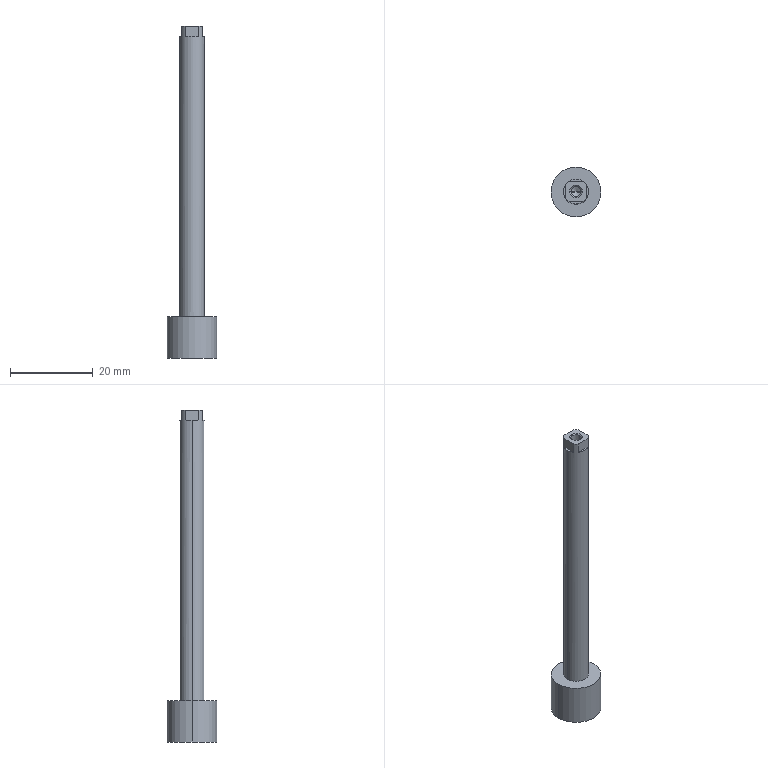Part | SolidWorks | features BaseBody 1 | 1 solid | 21 faces | box 12 x 12 x 80 mm | volume 3071 mm3 | plane 11 | cylinder 6 | cone 4 | commonest cylinder face diameters 2.459 x2 6 x2 12 x2
STEP:
#1=CARTESIAN_POINT('',(3.,0.,-37.5));
#2=VERTEX_POINT('',#1);
#3=CARTESIAN_POINT('',(-3.,0.,-37.5));
#4=VERTEX_POINT('',#3);
#5=CARTESIAN_POINT('',(0.,0.,-37.5));
#6=DIRECTION('',(0.,0.,1.));
#7=DIRECTION('',(1.,0.,0.));
#8=AXIS2_PLACEMENT_3D('',#5,#6,#7);
#9=CIRCLE('',#8,3.);
#10=EDGE_CURVE('',#2,#4,#9,.T.);
#11=ORIENTED_EDGE('',*,*,#10,.T.);
#12=CARTESIAN_POINT('',(-3.,0.,30.));
#13=VERTEX_POINT('',#12);
#14=CARTESIAN_POINT('',(-3.,0.,-2.5));
#15=DIRECTION('',(0.,0.,1.));
#16=VECTOR('',#15,1000.);
#17=LINE('',#14,#16);
#18=EDGE_CURVE('',#4,#13,#17,.T.);
#19=ORIENTED_EDGE('',*,*,#18,.T.);
#20=CARTESIAN_POINT('',(-2.5,1.658,30.));
#21=VERTEX_POINT('',#20);
#22=CARTESIAN_POINT('',(0.,0.,30.));
#23=DIRECTION('',(0.,0.,-1.));
#24=DIRECTION('',(1.,0.,0.));
#25=AXIS2_PLACEMENT_3D('',#22,#23,#24);
#26=CIRCLE('',#25,3.);
#27=EDGE_CURVE('',#13,#21,#26,.T.);
#28=ORIENTED_EDGE('',*,*,#27,.T.);
#29=CARTESIAN_POINT('',(-2.5,1.658,32.5));
#30=VERTEX_POINT('',#29);
#31=CARTESIAN_POINT('',(-2.5,1.658,-2.5));
#32=DIRECTION('',(0.,0.,1.));
#33=VECTOR('',#32,1000.);
#34=LINE('',#31,#33);
#35=EDGE_CURVE('',#21,#30,#34,.T.);
#36=ORIENTED_EDGE('',*,*,#35,.T.);
#37=CARTESIAN_POINT('',(-1.658,2.5,32.5));
#38=VERTEX_POINT('',#37);
#39=CARTESIAN_POINT('',(0.,0.,32.5));
#40=DIRECTION('',(0.,0.,1.));
#41=DIRECTION('',(1.,0.,0.));
#42=AXIS2_PLACEMENT_3D('',#39,#40,#41);
#43=CIRCLE('',#42,3.);
#44=EDGE_CURVE('',#38,#30,#43,.T.);
#45=ORIENTED_EDGE('',*,*,#44,.F.);
#46=CARTESIAN_POINT('',(-1.658,2.5,30.));
#47=VERTEX_POINT('',#46);
#48=CARTESIAN_POINT('',(-1.658,2.5,-2.5));
#49=DIRECTION('',(0.,0.,-1.));
#50=VECTOR('',#49,1000.);
#51=LINE('',#48,#50);
#52=EDGE_CURVE('',#38,#47,#51,.T.);
#53=ORIENTED_EDGE('',*,*,#52,.T.);
#54=CARTESIAN_POINT('',(1.658,2.5,30.));
#55=VERTEX_POINT('',#54);
#56=CARTESIAN_POINT('',(0.,0.,30.));
#57=DIRECTION('',(0.,0.,-1.));
#58=DIRECTION('',(1.,0.,0.));
#59=AXIS2_PLACEMENT_3D('',#56,#57,#58);
#60=CIRCLE('',#59,3.);
#61=EDGE_CURVE('',#47,#55,#60,.T.);
#62=ORIENTED_EDGE('',*,*,#61,.T.);
#63=CARTESIAN_POINT('',(1.658,2.5,32.5));
#64=VERTEX_POINT('',#63);
#65=CARTESIAN_POINT('',(1.658,2.5,-2.5));
#66=DIRECTION('',(0.,0.,1.));
#67=VECTOR('',#66,1000.);
#68=LINE('',#65,#67);
#69=EDGE_CURVE('',#55,#64,#68,.T.);
#70=ORIENTED_EDGE('',*,*,#69,.T.);
#71=CARTESIAN_POINT('',(2.5,1.658,32.5));
#72=VERTEX_POINT('',#71);
#73=CARTESIAN_POINT('',(0.,0.,32.5));
#74=DIRECTION('',(0.,0.,1.));
#75=DIRECTION('',(1.,0.,0.));
#76=AXIS2_PLACEMENT_3D('',#73,#74,#75);
#77=CIRCLE('',#76,3.);
#78=EDGE_CURVE('',#72,#64,#77,.T.);
#79=ORIENTED_EDGE('',*,*,#78,.F.);
#80=CARTESIAN_POINT('',(2.5,1.658,30.));
#81=VERTEX_POINT('',#80);
#82=CARTESIAN_POINT('',(2.5,1.658,-2.5));
#83=DIRECTION('',(0.,0.,-1.));
#84=VECTOR('',#83,1000.);
#85=LINE('',#82,#84);
#86=EDGE_CURVE('',#72,#81,#85,.T.);
#87=ORIENTED_EDGE('',*,*,#86,.T.);
#88=CARTESIAN_POINT('',(3.,0.,30.));
#89=VERTEX_POINT('',#88);
#90=CARTESIAN_POINT('',(0.,0.,30.));
#91=DIRECTION('',(0.,0.,-1.));
#92=DIRECTION('',(1.,0.,0.));
#93=AXIS2_PLACEMENT_3D('',#90,#91,#92);
#94=CIRCLE('',#93,3.);
#95=EDGE_CURVE('',#81,#89,#94,.T.);
#96=ORIENTED_EDGE('',*,*,#95,.T.);
#97=CARTESIAN_POINT('',(3.,0.,-2.5));
#98=DIRECTION('',(0.,0.,1.));
#99=VECTOR('',#98,1000.);
#100=LINE('',#97,#99);
#101=EDGE_CURVE('',#2,#89,#100,.T.);
#102=ORIENTED_EDGE('',*,*,#101,.F.);
#103=EDGE_LOOP('',(#11,#19,#28,#36,#45,#53,#62,#70,#79,#87,#96,#102));
#104=FACE_OUTER_BOUND('',#103,.T.);
#105=CARTESIAN_POINT('',(0.,0.,-2.5));
#106=DIRECTION('',(0.,0.,1.));
#107=DIRECTION('',(1.,0.,0.));
#108=AXIS2_PLACEMENT_3D('',#105,#106,#107);
#109=CYLINDRICAL_SURFACE('',#108,3.);
#110=ADVANCED_FACE('',(#104),#109,.T.);
#111=CARTESIAN_POINT('',(6.,0.,-47.5));
#112=VERTEX_POINT('',#111);
#113=CARTESIAN_POINT('',(-6.,0.,-47.5));
#114=VERTEX_POINT('',#113);
#115=CARTESIAN_POINT('',(0.,0.,-47.5));
#116=DIRECTION('',(0.,0.,1.));
#117=DIRECTION('',(1.,0.,0.));
#118=AXIS2_PLACEMENT_3D('',#115,#116,#117);
#119=CIRCLE('',#118,6.);
#120=EDGE_CURVE('',#112,#114,#119,.T.);
#121=ORIENTED_EDGE('',*,*,#120,.T.);
#122=CARTESIAN_POINT('',(-6.,0.,-37.5));
#123=VERTEX_POINT('',#122);
#124=CARTESIAN_POINT('',(-6.,0.,-42.5));
#125=DIRECTION('',(0.,0.,1.));
#126=VECTOR('',#125,1000.);
#127=LINE('',#124,#126);
#128=EDGE_CURVE('',#114,#123,#127,.T.);
#129=ORIENTED_EDGE('',*,*,#128,.T.);
#130=CARTESIAN_POINT('',(6.,0.,-37.5));
#131=VERTEX_POINT('',#130);
#132=CARTESIAN_POINT('',(0.,0.,-37.5));
#133=DIRECTION('',(0.,0.,1.));
#134=DIRECTION('',(1.,0.,0.));
#135=AXIS2_PLACEMENT_3D('',#132,#133,#134);
#136=CIRCLE('',#135,6.);
#137=EDGE_CURVE('',#131,#123,#136,.T.);
#138=ORIENTED_EDGE('',*,*,#137,.F.);
#139=CARTESIAN_POINT('',(6.,0.,-42.5));
#140=DIRECTION('',(0.,0.,1.));
#141=VECTOR('',#140,1000.);
#142=LINE('',#139,#141);
#143=EDGE_CURVE('',#112,#131,#142,.T.);
#144=ORIENTED_EDGE('',*,*,#143,.F.);
#145=EDGE_LOOP('',(#121,#129,#138,#144));
#146=FACE_OUTER_BOUND('',#145,.T.);
#147=CARTESIAN_POINT('',(0.,0.,-42.5));
#148=DIRECTION('',(0.,0.,1.));
#149=DIRECTION('',(1.,0.,0.));
#150=AXIS2_PLACEMENT_3D('',#147,#148,#149);
#151=CYLINDRICAL_SURFACE('',#150,6.);
#152=ADVANCED_FACE('',(#146),#151,.T.);
#153=CARTESIAN_POINT('',(-1.23,0.,32.23));
#154=VERTEX_POINT('',#153);
#155=CARTESIAN_POINT('',(1.23,0.,32.23));
#156=VERTEX_POINT('',#155);
#157=CARTESIAN_POINT('',(0.,0.,32.23));
#158=DIRECTION('',(0.,0.,1.));
#159=DIRECTION('',(1.,0.,0.));
#160=AXIS2_PLACEMENT_3D('',#157,#158,#159);
#161=CIRCLE('',#160,1.23);
#162=EDGE_CURVE('',#154,#156,#161,.T.);
#163=ORIENTED_EDGE('',*,*,#162,.F.);
#164=CARTESIAN_POINT('',(-1.5,0.,32.5));
#165=VERTEX_POINT('',#164);
#166=CARTESIAN_POINT('',(-1.5,0.,32.5));
#167=DIRECTION('',(-0.7071,0.,0.7071));
#168=VECTOR('',#167,1000.);
#169=LINE('',#166,#168);
#170=EDGE_CURVE('',#154,#165,#169,.T.);
#171=ORIENTED_EDGE('',*,*,#170,.T.);
#172=CARTESIAN_POINT('',(1.5,0.,32.5));
#173=VERTEX_POINT('',#172);
#174=CARTESIAN_POINT('',(0.,0.,32.5));
#175=DIRECTION('',(0.,0.,-1.));
#176=DIRECTION('',(1.,0.,0.));
#177=AXIS2_PLACEMENT_3D('',#174,#175,#176);
#178=CIRCLE('',#177,1.5);
#179=EDGE_CURVE('',#173,#165,#178,.T.);
#180=ORIENTED_EDGE('',*,*,#179,.F.);
#181=CARTESIAN_POINT('',(1.5,0.,32.5));
#182=DIRECTION('',(0.7071,0.,0.7071));
#183=VECTOR('',#182,1000.);
#184=LINE('',#181,#183);
#185=EDGE_CURVE('',#156,#173,#184,.T.);
#186=ORIENTED_EDGE('',*,*,#185,.F.);
#187=EDGE_LOOP('',(#163,#171,#180,#186));
#188=FACE_OUTER_BOUND('',#187,.T.);
#189=CARTESIAN_POINT('',(0.,0.,32.5));
#190=DIRECTION('',(0.,0.,1.));
#191=DIRECTION('',(1.,0.,0.));
#192=AXIS2_PLACEMENT_3D('',#189,#190,#191);
#193=CONICAL_SURFACE('',#192,1.5,0.7854);
#194=ADVANCED_FACE('',(#188),#193,.F.);
#195=CARTESIAN_POINT('',(-1.23,0.,27.));
#196=VERTEX_POINT('',#195);
#197=CARTESIAN_POINT('',(1.23,0.,27.));
#198=VERTEX_POINT('',#197);
#199=CARTESIAN_POINT('',(0.,0.,27.));
#200=DIRECTION('',(0.,0.,1.));
#201=DIRECTION('',(1.,0.,0.));
#202=AXIS2_PLACEMENT_3D('',#199,#200,#201);
#203=CIRCLE('',#202,1.23);
#204=EDGE_CURVE('',#196,#198,#203,.T.);
#205=ORIENTED_EDGE('',*,*,#204,.F.);
#206=CARTESIAN_POINT('',(-1.23,0.,29.615));
#207=DIRECTION('',(0.,0.,1.));
#208=VECTOR('',#207,1000.);
#209=LINE('',#206,#208);
#210=EDGE_CURVE('',#196,#154,#209,.T.);
#211=ORIENTED_EDGE('',*,*,#210,.T.);
#212=ORIENTED_EDGE('',*,*,#162,.T.);
#213=CARTESIAN_POINT('',(1.23,0.,29.615));
#214=DIRECTION('',(0.,0.,1.));
#215=VECTOR('',#214,1000.);
#216=LINE('',#213,#215);
#217=EDGE_CURVE('',#198,#156,#216,.T.);
#218=ORIENTED_EDGE('',*,*,#217,.F.);
#219=EDGE_LOOP('',(#205,#211,#212,#218));
#220=FACE_OUTER_BOUND('',#219,.T.);
#221=CARTESIAN_POINT('',(0.,0.,29.615));
#222=DIRECTION('',(0.,0.,1.));
#223=DIRECTION('',(1.,0.,0.));
#224=AXIS2_PLACEMENT_3D('',#221,#222,#223);
#225=CYLINDRICAL_SURFACE('',#224,1.23);
#226=ADVANCED_FACE('',(#220),#225,.F.);
#227=CARTESIAN_POINT('',(0.,0.,26.29));
#228=VERTEX_POINT('',#227);
#229=CARTESIAN_POINT('',(1.23,0.,27.));
#230=DIRECTION('',(0.866,0.,0.5));
#231=VECTOR('',#230,1000.);
#232=LINE('',#229,#231);
#233=EDGE_CURVE('',#228,#198,#232,.T.);
#234=ORIENTED_EDGE('',*,*,#233,.F.);
#235=CARTESIAN_POINT('',(-1.23,0.,27.));
#236=DIRECTION('',(-0.866,0.,0.5));
#237=VECTOR('',#236,1000.);
#238=LINE('',#235,#237);
#239=EDGE_CURVE('',#228,#196,#238,.T.);
#240=ORIENTED_EDGE('',*,*,#239,.T.);
#241=ORIENTED_EDGE('',*,*,#204,.T.);
#242=EDGE_LOOP('',(#234,#240,#241));
#243=FACE_OUTER_BOUND('',#242,.T.);
#244=CARTESIAN_POINT('',(0.,0.,27.));
#245=DIRECTION('',(0.,0.,1.));
#246=DIRECTION('',(1.,0.,0.));
#247=AXIS2_PLACEMENT_3D('',#244,#245,#246);
#248=CONICAL_SURFACE('',#247,1.23,1.047);
#249=ADVANCED_FACE('',(#243),#248,.F.);
#250=ORIENTED_EDGE('',*,*,#18,.F.);
#251=CARTESIAN_POINT('',(0.,0.,-37.5));
#252=DIRECTION('',(0.,0.,1.));
#253=DIRECTION('',(1.,0.,0.));
#254=AXIS2_PLACEMENT_3D('',#251,#252,#253);
#255=CIRCLE('',#254,3.);
#256=EDGE_CURVE('',#4,#2,#255,.T.);
#257=ORIENTED_EDGE('',*,*,#256,.T.);
#258=ORIENTED_EDGE('',*,*,#101,.T.);
#259=CARTESIAN_POINT('',(2.5,-1.658,30.));
#260=VERTEX_POINT('',#259);
#261=CARTESIAN_POINT('',(0.,0.,30.));
#262=DIRECTION('',(0.,0.,-1.));
#263=DIRECTION('',(1.,0.,0.));
#264=AXIS2_PLACEMENT_3D('',#261,#262,#263);
#265=CIRCLE('',#264,3.);
#266=EDGE_CURVE('',#89,#260,#265,.T.);
#267=ORIENTED_EDGE('',*,*,#266,.T.);
#268=CARTESIAN_POINT('',(2.5,-1.658,32.5));
#269=VERTEX_POINT('',#268);
#270=CARTESIAN_POINT('',(2.5,-1.658,-2.5));
#271=DIRECTION('',(0.,0.,1.));
#272=VECTOR('',#271,1000.);
#273=LINE('',#270,#272);
#274=EDGE_CURVE('',#260,#269,#273,.T.);
#275=ORIENTED_EDGE('',*,*,#274,.T.);
#276=CARTESIAN_POINT('',(1.658,-2.5,32.5));
#277=VERTEX_POINT('',#276);
#278=CARTESIAN_POINT('',(0.,0.,32.5));
#279=DIRECTION('',(0.,0.,1.));
#280=DIRECTION('',(1.,0.,0.));
#281=AXIS2_PLACEMENT_3D('',#278,#279,#280);
#282=CIRCLE('',#281,3.);
#283=EDGE_CURVE('',#277,#269,#282,.T.);
#284=ORIENTED_EDGE('',*,*,#283,.F.);
#285=CARTESIAN_POINT('',(1.658,-2.5,30.));
#286=VERTEX_POINT('',#285);
#287=CARTESIAN_POINT('',(1.658,-2.5,-2.5));
#288=DIRECTION('',(0.,0.,-1.));
#289=VECTOR('',#288,1000.);
#290=LINE('',#287,#289);
#291=EDGE_CURVE('',#277,#286,#290,.T.);
#292=ORIENTED_EDGE('',*,*,#291,.T.);
#293=CARTESIAN_POINT('',(-1.658,-2.5,30.));
#294=VERTEX_POINT('',#293);
#295=CARTESIAN_POINT('',(0.,0.,30.));
#296=DIRECTION('',(0.,0.,-1.));
#297=DIRECTION('',(1.,0.,0.));
#298=AXIS2_PLACEMENT_3D('',#295,#296,#297);
#299=CIRCLE('',#298,3.);
#300=EDGE_CURVE('',#286,#294,#299,.T.);
#301=ORIENTED_EDGE('',*,*,#300,.T.);
#302=CARTESIAN_POINT('',(-1.658,-2.5,32.5));
#303=VERTEX_POINT('',#302);
#304=CARTESIAN_POINT('',(-1.658,-2.5,-2.5));
#305=DIRECTION('',(0.,0.,1.));
#306=VECTOR('',#305,1000.);
#307=LINE('',#304,#306);
#308=EDGE_CURVE('',#294,#303,#307,.T.);
#309=ORIENTED_EDGE('',*,*,#308,.T.);
#310=CARTESIAN_POINT('',(-2.5,-1.658,32.5));
#311=VERTEX_POINT('',#310);
#312=CARTESIAN_POINT('',(0.,0.,32.5));
#313=DIRECTION('',(0.,0.,1.));
#314=DIRECTION('',(1.,0.,0.));
#315=AXIS2_PLACEMENT_3D('',#312,#313,#314);
#316=CIRCLE('',#315,3.);
#317=EDGE_CURVE('',#311,#303,#316,.T.);
#318=ORIENTED_EDGE('',*,*,#317,.F.);
#319=CARTESIAN_POINT('',(-2.5,-1.658,30.));
#320=VERTEX_POINT('',#319);
#321=CARTESIAN_POINT('',(-2.5,-1.658,-2.5));
#322=DIRECTION('',(0.,0.,-1.));
#323=VECTOR('',#322,1000.);
#324=LINE('',#321,#323);
#325=EDGE_CURVE('',#311,#320,#324,.T.);
#326=ORIENTED_EDGE('',*,*,#325,.T.);
#327=CARTESIAN_POINT('',(0.,0.,30.));
#328=DIRECTION('',(0.,0.,-1.));
#329=DIRECTION('',(1.,0.,0.));
#330=AXIS2_PLACEMENT_3D('',#327,#328,#329);
#331=CIRCLE('',#330,3.);
#332=EDGE_CURVE('',#320,#13,#331,.T.);
#333=ORIENTED_EDGE('',*,*,#332,.T.);
#334=EDGE_LOOP('',(#250,#257,#258,#267,#275,#284,#292,#301,#309,#318,#326,#333));
#335=FACE_OUTER_BOUND('',#334,.T.);
#336=CARTESIAN_POINT('',(0.,0.,-2.5));
#337=DIRECTION('',(0.,0.,1.));
#338=DIRECTION('',(1.,0.,0.));
#339=AXIS2_PLACEMENT_3D('',#336,#337,#338);
#340=CYLINDRICAL_SURFACE('',#339,3.);
#341=ADVANCED_FACE('',(#335),#340,.T.);
#342=ORIENTED_EDGE('',*,*,#10,.F.);
#343=ORIENTED_EDGE('',*,*,#256,.F.);
#344=EDGE_LOOP('',(#342,#343));
#345=FACE_BOUND('',#344,.T.);
#346=ORIENTED_EDGE('',*,*,#137,.T.);
#347=CARTESIAN_POINT('',(0.,0.,-37.5));
#348=DIRECTION('',(0.,0.,1.));
#349=DIRECTION('',(1.,0.,0.));
#350=AXIS2_PLACEMENT_3D('',#347,#348,#349);
#351=CIRCLE('',#350,6.);
#352=EDGE_CURVE('',#123,#131,#351,.T.);
#353=ORIENTED_EDGE('',*,*,#352,.T.);
#354=EDGE_LOOP('',(#346,#353));
#355=FACE_OUTER_BOUND('',#354,.T.);
#356=CARTESIAN_POINT('',(4.5,0.,-37.5));
#357=DIRECTION('',(0.,0.,1.));
#358=DIRECTION('',(1.,0.,0.));
#359=AXIS2_PLACEMENT_3D('',#356,#357,#358);
#360=PLANE('',#359);
#361=ADVANCED_FACE('',(#345,#355),#360,.T.);
#362=CARTESIAN_POINT('',(-2.5,0.,30.));
#363=DIRECTION('',(0.,1.,0.));
#364=VECTOR('',#363,1000.);
#365=LINE('',#362,#364);
#366=EDGE_CURVE('',#320,#21,#365,.T.);
#367=ORIENTED_EDGE('',*,*,#366,.T.);
#368=ORIENTED_EDGE('',*,*,#27,.F.);
#369=ORIENTED_EDGE('',*,*,#332,.F.);
#370=EDGE_LOOP('',(#367,#368,#369));
#371=FACE_OUTER_BOUND('',#370,.T.);
#372=CARTESIAN_POINT('',(0.,0.,30.));
#373=DIRECTION('',(0.,0.,1.));
#374=DIRECTION('',(1.,0.,0.));
#375=AXIS2_PLACEMENT_3D('',#372,#373,#374);
#376=PLANE('',#375);
#377=ADVANCED_FACE('',(#371),#376,.T.);
#378=CARTESIAN_POINT('',(-2.5,-2.5,32.5));
#379=DIRECTION('',(0.,-1.,0.));
#380=VECTOR('',#379,1000.);
#381=LINE('',#378,#380);
#382=EDGE_CURVE('',#30,#311,#381,.T.);
#383=ORIENTED_EDGE('',*,*,#382,.F.);
#384=ORIENTED_EDGE('',*,*,#35,.F.);
#385=ORIENTED_EDGE('',*,*,#366,.F.);
#386=ORIENTED_EDGE('',*,*,#325,.F.);
#387=EDGE_LOOP('',(#383,#384,#385,#386));
#388=FACE_OUTER_BOUND('',#387,.T.);
#389=CARTESIAN_POINT('',(-2.5,-2.5,32.5));
#390=DIRECTION('',(1.,0.,0.));
#391=DIRECTION('',(0.,0.,-1.));
#392=AXIS2_PLACEMENT_3D('',#389,#390,#391);
#393=PLANE('',#392);
#394=ADVANCED_FACE('',(#388),#393,.F.);
#395=CARTESIAN_POINT('',(2.5,-2.5,32.5));
#396=DIRECTION('',(1.,0.,0.));
#397=VECTOR('',#396,1000.);
#398=LINE('',#395,#397);
#399=EDGE_CURVE('',#303,#277,#398,.T.);
#400=ORIENTED_EDGE('',*,*,#399,.F.);
#401=ORIENTED_EDGE('',*,*,#308,.F.);
#402=CARTESIAN_POINT('',(2.5,-2.5,30.));
#403=DIRECTION('',(-1.,0.,0.));
#404=VECTOR('',#403,1000.);
#405=LINE('',#402,#404);
#406=EDGE_CURVE('',#286,#294,#405,.T.);
#407=ORIENTED_EDGE('',*,*,#406,.F.);
#408=ORIENTED_EDGE('',*,*,#291,.F.);
#409=EDGE_LOOP('',(#400,#401,#407,#408));
#410=FACE_OUTER_BOUND('',#409,.T.);
#411=CARTESIAN_POINT('',(2.5,-2.5,32.5));
#412=DIRECTION('',(0.,1.,0.));
#413=DIRECTION('',(0.,0.,1.));
#414=AXIS2_PLACEMENT_3D('',#411,#412,#413);
#415=PLANE('',#414);
#416=ADVANCED_FACE('',(#410),#415,.F.);
#417=ORIENTED_EDGE('',*,*,#300,.F.);
#418=ORIENTED_EDGE('',*,*,#406,.T.);
#419=EDGE_LOOP('',(#417,#418));
#420=FACE_OUTER_BOUND('',#419,.T.);
#421=CARTESIAN_POINT('',(0.,0.,30.));
#422=DIRECTION('',(0.,0.,1.));
#423=DIRECTION('',(1.,0.,0.));
#424=AXIS2_PLACEMENT_3D('',#421,#422,#423);
#425=PLANE('',#424);
#426=ADVANCED_FACE('',(#420),#425,.T.);
#427=CARTESIAN_POINT('',(2.5,2.5,32.5));
#428=DIRECTION('',(0.,1.,0.));
#429=VECTOR('',#428,1000.);
#430=LINE('',#427,#429);
#431=EDGE_CURVE('',#269,#72,#430,.T.);
#432=ORIENTED_EDGE('',*,*,#431,.F.);
#433=ORIENTED_EDGE('',*,*,#274,.F.);
#434=CARTESIAN_POINT('',(2.5,2.5,30.));
#435=DIRECTION('',(0.,-1.,0.));
#436=VECTOR('',#435,1000.);
#437=LINE('',#434,#436);
#438=EDGE_CURVE('',#81,#260,#437,.T.);
#439=ORIENTED_EDGE('',*,*,#438,.F.);
#440=ORIENTED_EDGE('',*,*,#86,.F.);
#441=EDGE_LOOP('',(#432,#433,#439,#440));
#442=FACE_OUTER_BOUND('',#441,.T.);
#443=CARTESIAN_POINT('',(2.5,2.5,32.5));
#444=DIRECTION('',(-1.,0.,0.));
#445=DIRECTION('',(0.,0.,1.));
#446=AXIS2_PLACEMENT_3D('',#443,#444,#445);
#447=PLANE('',#446);
#448=ADVANCED_FACE('',(#442),#447,.F.);
#449=ORIENTED_EDGE('',*,*,#438,.T.);
#450=ORIENTED_EDGE('',*,*,#266,.F.);
#451=ORIENTED_EDGE('',*,*,#95,.F.);
#452=EDGE_LOOP('',(#449,#450,#451));
#453=FACE_OUTER_BOUND('',#452,.T.);
#454=CARTESIAN_POINT('',(0.,0.,30.));
#455=DIRECTION('',(0.,0.,1.));
#456=DIRECTION('',(1.,0.,0.));
#457=AXIS2_PLACEMENT_3D('',#454,#455,#456);
#458=PLANE('',#457);
#459=ADVANCED_FACE('',(#453),#458,.T.);
#460=ORIENTED_EDGE('',*,*,#128,.F.);
#461=CARTESIAN_POINT('',(0.,0.,-47.5));
#462=DIRECTION('',(0.,0.,1.));
#463=DIRECTION('',(1.,0.,0.));
#464=AXIS2_PLACEMENT_3D('',#461,#462,#463);
#465=CIRCLE('',#464,6.);
#466=EDGE_CURVE('',#114,#112,#465,.T.);
#467=ORIENTED_EDGE('',*,*,#466,.T.);
#468=ORIENTED_EDGE('',*,*,#143,.T.);
#469=ORIENTED_EDGE('',*,*,#352,.F.);
#470=EDGE_LOOP('',(#460,#467,#468,#469));
#471=FACE_OUTER_BOUND('',#470,.T.);
#472=CARTESIAN_POINT('',(0.,0.,-42.5));
#473=DIRECTION('',(0.,0.,1.));
#474=DIRECTION('',(1.,0.,0.));
#475=AXIS2_PLACEMENT_3D('',#472,#473,#474);
#476=CYLINDRICAL_SURFACE('',#475,6.);
#477=ADVANCED_FACE('',(#471),#476,.T.);
#478=CARTESIAN_POINT('',(-2.5,2.5,32.5));
#479=DIRECTION('',(-1.,0.,0.));
#480=VECTOR('',#479,1000.);
#481=LINE('',#478,#480);
#482=EDGE_CURVE('',#64,#38,#481,.T.);
#483=ORIENTED_EDGE('',*,*,#482,.F.);
#484=ORIENTED_EDGE('',*,*,#69,.F.);
#485=CARTESIAN_POINT('',(-2.5,2.5,30.));
#486=DIRECTION('',(1.,0.,0.));
#487=VECTOR('',#486,1000.);
#488=LINE('',#485,#487);
#489=EDGE_CURVE('',#47,#55,#488,.T.);
#490=ORIENTED_EDGE('',*,*,#489,.F.);
#491=ORIENTED_EDGE('',*,*,#52,.F.);
#492=EDGE_LOOP('',(#483,#484,#490,#491));
#493=FACE_OUTER_BOUND('',#492,.T.);
#494=CARTESIAN_POINT('',(-2.5,2.5,32.5));
#495=DIRECTION('',(0.,-1.,0.));
#496=DIRECTION('',(0.,0.,-1.));
#497=AXIS2_PLACEMENT_3D('',#494,#495,#496);
#498=PLANE('',#497);
#499=ADVANCED_FACE('',(#493),#498,.F.);
#500=ORIENTED_EDGE('',*,*,#61,.F.);
#501=ORIENTED_EDGE('',*,*,#489,.T.);
#502=EDGE_LOOP('',(#500,#501));
#503=FACE_OUTER_BOUND('',#502,.T.);
#504=CARTESIAN_POINT('',(0.,0.,30.));
#505=DIRECTION('',(0.,0.,1.));
#506=DIRECTION('',(1.,0.,0.));
#507=AXIS2_PLACEMENT_3D('',#504,#505,#506);
#508=PLANE('',#507);
#509=ADVANCED_FACE('',(#503),#508,.T.);
#510=ORIENTED_EDGE('',*,*,#179,.T.);
#511=CARTESIAN_POINT('',(0.,0.,32.5));
#512=DIRECTION('',(0.,0.,-1.));
#513=DIRECTION('',(1.,0.,0.));
#514=AXIS2_PLACEMENT_3D('',#511,#512,#513);
#515=CIRCLE('',#514,1.5);
#516=EDGE_CURVE('',#165,#173,#515,.T.);
#517=ORIENTED_EDGE('',*,*,#516,.T.);
#518=EDGE_LOOP('',(#510,#517));
#519=FACE_BOUND('',#518,.T.);
#520=ORIENTED_EDGE('',*,*,#431,.T.);
#521=ORIENTED_EDGE('',*,*,#78,.T.);
#522=ORIENTED_EDGE('',*,*,#482,.T.);
#523=ORIENTED_EDGE('',*,*,#44,.T.);
#524=ORIENTED_EDGE('',*,*,#382,.T.);
#525=ORIENTED_EDGE('',*,*,#317,.T.);
#526=ORIENTED_EDGE('',*,*,#399,.T.);
#527=ORIENTED_EDGE('',*,*,#283,.T.);
#528=EDGE_LOOP('',(#520,#521,#522,#523,#524,#525,#526,#527));
#529=FACE_OUTER_BOUND('',#528,.T.);
#530=CARTESIAN_POINT('',(2.25,0.,32.5));
#531=DIRECTION('',(0.,0.,1.));
#532=DIRECTION('',(1.,0.,0.));
#533=AXIS2_PLACEMENT_3D('',#530,#531,#532);
#534=PLANE('',#533);
#535=ADVANCED_FACE('',(#519,#529),#534,.T.);
#536=ORIENTED_EDGE('',*,*,#120,.F.);
#537=ORIENTED_EDGE('',*,*,#466,.F.);
#538=EDGE_LOOP('',(#536,#537));
#539=FACE_OUTER_BOUND('',#538,.T.);
#540=CARTESIAN_POINT('',(3.,0.,-47.5));
#541=DIRECTION('',(0.,0.,-1.));
#542=DIRECTION('',(-1.,0.,0.));
#543=AXIS2_PLACEMENT_3D('',#540,#541,#542);
#544=PLANE('',#543);
#545=ADVANCED_FACE('',(#539),#544,.T.);
#546=ORIENTED_EDGE('',*,*,#170,.F.);
#547=CARTESIAN_POINT('',(0.,0.,32.23));
#548=DIRECTION('',(0.,0.,1.));
#549=DIRECTION('',(1.,0.,0.));
#550=AXIS2_PLACEMENT_3D('',#547,#548,#549);
#551=CIRCLE('',#550,1.23);
#552=EDGE_CURVE('',#156,#154,#551,.T.);
#553=ORIENTED_EDGE('',*,*,#552,.F.);
#554=ORIENTED_EDGE('',*,*,#185,.T.);
#555=ORIENTED_EDGE('',*,*,#516,.F.);
#556=EDGE_LOOP('',(#546,#553,#554,#555));
#557=FACE_OUTER_BOUND('',#556,.T.);
#558=CARTESIAN_POINT('',(0.,0.,32.5));
#559=DIRECTION('',(0.,0.,1.));
#560=DIRECTION('',(1.,0.,0.));
#561=AXIS2_PLACEMENT_3D('',#558,#559,#560);
#562=CONICAL_SURFACE('',#561,1.5,0.7854);
#563=ADVANCED_FACE('',(#557),#562,.F.);
#564=ORIENTED_EDGE('',*,*,#210,.F.);
#565=CARTESIAN_POINT('',(0.,0.,27.));
#566=DIRECTION('',(0.,0.,1.));
#567=DIRECTION('',(1.,0.,0.));
#568=AXIS2_PLACEMENT_3D('',#565,#566,#567);
#569=CIRCLE('',#568,1.23);
#570=EDGE_CURVE('',#198,#196,#569,.T.);
#571=ORIENTED_EDGE('',*,*,#570,.F.);
#572=ORIENTED_EDGE('',*,*,#217,.T.);
#573=ORIENTED_EDGE('',*,*,#552,.T.);
#574=EDGE_LOOP('',(#564,#571,#572,#573));
#575=FACE_OUTER_BOUND('',#574,.T.);
#576=CARTESIAN_POINT('',(0.,0.,29.615));
#577=DIRECTION('',(0.,0.,1.));
#578=DIRECTION('',(1.,0.,0.));
#579=AXIS2_PLACEMENT_3D('',#576,#577,#578);
#580=CYLINDRICAL_SURFACE('',#579,1.23);
#581=ADVANCED_FACE('',(#575),#580,.F.);
#582=ORIENTED_EDGE('',*,*,#239,.F.);
#583=ORIENTED_EDGE('',*,*,#233,.T.);
#584=ORIENTED_EDGE('',*,*,#570,.T.);
#585=EDGE_LOOP('',(#582,#583,#584));
#586=FACE_OUTER_BOUND('',#585,.T.);
#587=CARTESIAN_POINT('',(0.,0.,27.));
#588=DIRECTION('',(0.,0.,1.));
#589=DIRECTION('',(1.,0.,0.));
#590=AXIS2_PLACEMENT_3D('',#587,#588,#589);
#591=CONICAL_SURFACE('',#590,1.23,1.047);
#592=ADVANCED_FACE('',(#586),#591,.F.);
#593=CLOSED_SHELL('',(#110,#152,#194,#226,#249,#341,#361,#377,#394,#416,#426,#448,#459,#477,#499,#509,#535,#545,#563,#581,#592));
#594=MANIFOLD_SOLID_BREP('',#593);
#595=CARTESIAN_POINT('',(0.,0.,0.));
#596=DIRECTION('',(0.,0.,1.));
#597=DIRECTION('',(1.,0.,0.));
#598=AXIS2_PLACEMENT_3D('',#595,#596,#597);
#599=(LENGTH_UNIT()NAMED_UNIT(*)SI_UNIT(.MILLI.,.METRE.));
#600=UNCERTAINTY_MEASURE_WITH_UNIT(LENGTH_MEASURE(0.00001),#599,'','');
#601=(NAMED_UNIT(*)PLANE_ANGLE_UNIT()SI_UNIT($,.RADIAN.));
#602=(NAMED_UNIT(*)SI_UNIT($,.STERADIAN.)SOLID_ANGLE_UNIT());
#603=(GEOMETRIC_REPRESENTATION_CONTEXT(3)GLOBAL_UNCERTAINTY_ASSIGNED_CONTEXT((#600))GLOBAL_UNIT_ASSIGNED_CONTEXT((#599,#601,#602))REPRESENTATION_CONTEXT('',''));
#604=ADVANCED_BREP_SHAPE_REPRESENTATION('',(#594,#598),#603);